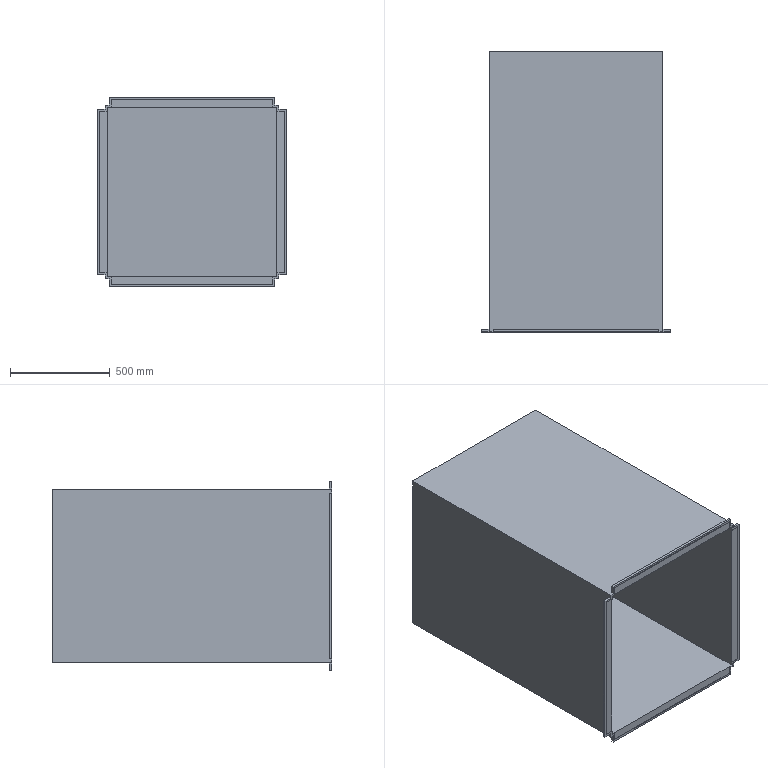Part | SolidWorks | features CirPattern 1, Extrusion 1, ICE 1, RefAxis 1, Shell 1 | 1 solid | 43 faces | box 950 x 1400 x 950 mm | volume 61176455 mm3 | plane 43
STEP:
#1=CARTESIAN_POINT('',(-435.,12.,-415.));
#2=VERTEX_POINT('',#1);
#3=CARTESIAN_POINT('',(-435.,0.,-415.));
#4=VERTEX_POINT('',#3);
#5=CARTESIAN_POINT('',(-435.,1400.,-415.));
#6=DIRECTION('',(0.,-1.,0.));
#7=VECTOR('',#6,1000.);
#8=LINE('',#5,#7);
#9=EDGE_CURVE('',#2,#4,#8,.T.);
#10=ORIENTED_EDGE('',*,*,#9,.F.);
#11=CARTESIAN_POINT('',(-435.,12.,415.));
#12=VERTEX_POINT('',#11);
#13=CARTESIAN_POINT('',(-435.,12.,435.));
#14=DIRECTION('',(0.,0.,-1.));
#15=VECTOR('',#14,1000.);
#16=LINE('',#13,#15);
#17=EDGE_CURVE('',#12,#2,#16,.T.);
#18=ORIENTED_EDGE('',*,*,#17,.F.);
#19=CARTESIAN_POINT('',(-435.,0.,415.));
#20=VERTEX_POINT('',#19);
#21=CARTESIAN_POINT('',(-435.,1400.,415.));
#22=DIRECTION('',(0.,1.,0.));
#23=VECTOR('',#22,1000.);
#24=LINE('',#21,#23);
#25=EDGE_CURVE('',#20,#12,#24,.T.);
#26=ORIENTED_EDGE('',*,*,#25,.F.);
#27=CARTESIAN_POINT('',(-435.,0.,435.));
#28=VERTEX_POINT('',#27);
#29=CARTESIAN_POINT('',(-435.,0.,435.));
#30=DIRECTION('',(0.,0.,1.));
#31=VECTOR('',#30,1000.);
#32=LINE('',#29,#31);
#33=EDGE_CURVE('',#20,#28,#32,.T.);
#34=ORIENTED_EDGE('',*,*,#33,.T.);
#35=CARTESIAN_POINT('',(-435.,1400.,435.));
#36=VERTEX_POINT('',#35);
#37=CARTESIAN_POINT('',(-435.,1400.,435.));
#38=DIRECTION('',(0.,-1.,0.));
#39=VECTOR('',#38,1000.);
#40=LINE('',#37,#39);
#41=EDGE_CURVE('',#36,#28,#40,.T.);
#42=ORIENTED_EDGE('',*,*,#41,.F.);
#43=CARTESIAN_POINT('',(-435.,1400.,-435.));
#44=VERTEX_POINT('',#43);
#45=CARTESIAN_POINT('',(-435.,1400.,435.));
#46=DIRECTION('',(0.,0.,1.));
#47=VECTOR('',#46,1000.);
#48=LINE('',#45,#47);
#49=EDGE_CURVE('',#44,#36,#48,.T.);
#50=ORIENTED_EDGE('',*,*,#49,.F.);
#51=CARTESIAN_POINT('',(-435.,0.,-435.));
#52=VERTEX_POINT('',#51);
#53=CARTESIAN_POINT('',(-435.,1400.,-435.));
#54=DIRECTION('',(0.,-1.,0.));
#55=VECTOR('',#54,1000.);
#56=LINE('',#53,#55);
#57=EDGE_CURVE('',#44,#52,#56,.T.);
#58=ORIENTED_EDGE('',*,*,#57,.T.);
#59=CARTESIAN_POINT('',(-435.,0.,435.));
#60=DIRECTION('',(0.,0.,1.));
#61=VECTOR('',#60,1000.);
#62=LINE('',#59,#61);
#63=EDGE_CURVE('',#52,#4,#62,.T.);
#64=ORIENTED_EDGE('',*,*,#63,.T.);
#65=EDGE_LOOP('',(#10,#18,#26,#34,#42,#50,#58,#64));
#66=FACE_OUTER_BOUND('',#65,.T.);
#67=CARTESIAN_POINT('',(-435.,1400.,435.));
#68=DIRECTION('',(1.,0.,0.));
#69=DIRECTION('',(0.,0.,-1.));
#70=AXIS2_PLACEMENT_3D('',#67,#68,#69);
#71=PLANE('',#70);
#72=ADVANCED_FACE('',(#66),#71,.F.);
#73=CARTESIAN_POINT('',(435.,0.,-415.));
#74=VERTEX_POINT('',#73);
#75=CARTESIAN_POINT('',(435.,12.,-415.));
#76=VERTEX_POINT('',#75);
#77=CARTESIAN_POINT('',(435.,1400.,-415.));
#78=DIRECTION('',(0.,1.,0.));
#79=VECTOR('',#78,1000.);
#80=LINE('',#77,#79);
#81=EDGE_CURVE('',#74,#76,#80,.T.);
#82=ORIENTED_EDGE('',*,*,#81,.F.);
#83=CARTESIAN_POINT('',(435.,0.,-435.));
#84=VERTEX_POINT('',#83);
#85=CARTESIAN_POINT('',(435.,0.,435.));
#86=DIRECTION('',(0.,0.,-1.));
#87=VECTOR('',#86,1000.);
#88=LINE('',#85,#87);
#89=EDGE_CURVE('',#74,#84,#88,.T.);
#90=ORIENTED_EDGE('',*,*,#89,.T.);
#91=CARTESIAN_POINT('',(435.,1400.,-435.));
#92=VERTEX_POINT('',#91);
#93=CARTESIAN_POINT('',(435.,1400.,-435.));
#94=DIRECTION('',(0.,-1.,0.));
#95=VECTOR('',#94,1000.);
#96=LINE('',#93,#95);
#97=EDGE_CURVE('',#92,#84,#96,.T.);
#98=ORIENTED_EDGE('',*,*,#97,.F.);
#99=CARTESIAN_POINT('',(435.,1400.,435.));
#100=VERTEX_POINT('',#99);
#101=CARTESIAN_POINT('',(435.,1400.,435.));
#102=DIRECTION('',(0.,0.,-1.));
#103=VECTOR('',#102,1000.);
#104=LINE('',#101,#103);
#105=EDGE_CURVE('',#100,#92,#104,.T.);
#106=ORIENTED_EDGE('',*,*,#105,.F.);
#107=CARTESIAN_POINT('',(435.,0.,435.));
#108=VERTEX_POINT('',#107);
#109=CARTESIAN_POINT('',(435.,1400.,435.));
#110=DIRECTION('',(0.,-1.,0.));
#111=VECTOR('',#110,1000.);
#112=LINE('',#109,#111);
#113=EDGE_CURVE('',#100,#108,#112,.T.);
#114=ORIENTED_EDGE('',*,*,#113,.T.);
#115=CARTESIAN_POINT('',(435.,0.,415.));
#116=VERTEX_POINT('',#115);
#117=CARTESIAN_POINT('',(435.,0.,435.));
#118=DIRECTION('',(0.,0.,-1.));
#119=VECTOR('',#118,1000.);
#120=LINE('',#117,#119);
#121=EDGE_CURVE('',#108,#116,#120,.T.);
#122=ORIENTED_EDGE('',*,*,#121,.T.);
#123=CARTESIAN_POINT('',(435.,12.,415.));
#124=VERTEX_POINT('',#123);
#125=CARTESIAN_POINT('',(435.,1400.,415.));
#126=DIRECTION('',(0.,-1.,0.));
#127=VECTOR('',#126,1000.);
#128=LINE('',#125,#127);
#129=EDGE_CURVE('',#124,#116,#128,.T.);
#130=ORIENTED_EDGE('',*,*,#129,.F.);
#131=CARTESIAN_POINT('',(435.,12.,435.));
#132=DIRECTION('',(0.,0.,1.));
#133=VECTOR('',#132,1000.);
#134=LINE('',#131,#133);
#135=EDGE_CURVE('',#76,#124,#134,.T.);
#136=ORIENTED_EDGE('',*,*,#135,.F.);
#137=EDGE_LOOP('',(#82,#90,#98,#106,#114,#122,#130,#136));
#138=FACE_OUTER_BOUND('',#137,.T.);
#139=CARTESIAN_POINT('',(435.,1400.,435.));
#140=DIRECTION('',(-1.,0.,0.));
#141=DIRECTION('',(0.,0.,1.));
#142=AXIS2_PLACEMENT_3D('',#139,#140,#141);
#143=PLANE('',#142);
#144=ADVANCED_FACE('',(#138),#143,.F.);
#145=CARTESIAN_POINT('',(-415.,0.,-435.));
#146=VERTEX_POINT('',#145);
#147=CARTESIAN_POINT('',(-415.,12.,-435.));
#148=VERTEX_POINT('',#147);
#149=CARTESIAN_POINT('',(-415.,1400.,-435.));
#150=DIRECTION('',(0.,1.,0.));
#151=VECTOR('',#150,1000.);
#152=LINE('',#149,#151);
#153=EDGE_CURVE('',#146,#148,#152,.T.);
#154=ORIENTED_EDGE('',*,*,#153,.F.);
#155=CARTESIAN_POINT('',(435.,0.,-435.));
#156=DIRECTION('',(-1.,0.,0.));
#157=VECTOR('',#156,1000.);
#158=LINE('',#155,#157);
#159=EDGE_CURVE('',#146,#52,#158,.T.);
#160=ORIENTED_EDGE('',*,*,#159,.T.);
#161=ORIENTED_EDGE('',*,*,#57,.F.);
#162=CARTESIAN_POINT('',(435.,1400.,-435.));
#163=DIRECTION('',(-1.,0.,0.));
#164=VECTOR('',#163,1000.);
#165=LINE('',#162,#164);
#166=EDGE_CURVE('',#92,#44,#165,.T.);
#167=ORIENTED_EDGE('',*,*,#166,.F.);
#168=ORIENTED_EDGE('',*,*,#97,.T.);
#169=CARTESIAN_POINT('',(415.,0.,-435.));
#170=VERTEX_POINT('',#169);
#171=CARTESIAN_POINT('',(435.,0.,-435.));
#172=DIRECTION('',(-1.,0.,0.));
#173=VECTOR('',#172,1000.);
#174=LINE('',#171,#173);
#175=EDGE_CURVE('',#84,#170,#174,.T.);
#176=ORIENTED_EDGE('',*,*,#175,.T.);
#177=CARTESIAN_POINT('',(415.,12.,-435.));
#178=VERTEX_POINT('',#177);
#179=CARTESIAN_POINT('',(415.,1400.,-435.));
#180=DIRECTION('',(0.,-1.,0.));
#181=VECTOR('',#180,1000.);
#182=LINE('',#179,#181);
#183=EDGE_CURVE('',#178,#170,#182,.T.);
#184=ORIENTED_EDGE('',*,*,#183,.F.);
#185=CARTESIAN_POINT('',(435.,12.,-435.));
#186=DIRECTION('',(1.,0.,0.));
#187=VECTOR('',#186,1000.);
#188=LINE('',#185,#187);
#189=EDGE_CURVE('',#148,#178,#188,.T.);
#190=ORIENTED_EDGE('',*,*,#189,.F.);
#191=EDGE_LOOP('',(#154,#160,#161,#167,#168,#176,#184,#190));
#192=FACE_OUTER_BOUND('',#191,.T.);
#193=CARTESIAN_POINT('',(435.,1400.,-435.));
#194=DIRECTION('',(0.,0.,1.));
#195=DIRECTION('',(1.,0.,0.));
#196=AXIS2_PLACEMENT_3D('',#193,#194,#195);
#197=PLANE('',#196);
#198=ADVANCED_FACE('',(#192),#197,.F.);
#199=CARTESIAN_POINT('',(-415.,12.,435.));
#200=VERTEX_POINT('',#199);
#201=CARTESIAN_POINT('',(-415.,0.,435.));
#202=VERTEX_POINT('',#201);
#203=CARTESIAN_POINT('',(-415.,1400.,435.));
#204=DIRECTION('',(0.,-1.,0.));
#205=VECTOR('',#204,1000.);
#206=LINE('',#203,#205);
#207=EDGE_CURVE('',#200,#202,#206,.T.);
#208=ORIENTED_EDGE('',*,*,#207,.F.);
#209=CARTESIAN_POINT('',(415.,12.,435.));
#210=VERTEX_POINT('',#209);
#211=CARTESIAN_POINT('',(435.,12.,435.));
#212=DIRECTION('',(-1.,0.,0.));
#213=VECTOR('',#212,1000.);
#214=LINE('',#211,#213);
#215=EDGE_CURVE('',#210,#200,#214,.T.);
#216=ORIENTED_EDGE('',*,*,#215,.F.);
#217=CARTESIAN_POINT('',(415.,0.,435.));
#218=VERTEX_POINT('',#217);
#219=CARTESIAN_POINT('',(415.,1400.,435.));
#220=DIRECTION('',(0.,1.,0.));
#221=VECTOR('',#220,1000.);
#222=LINE('',#219,#221);
#223=EDGE_CURVE('',#218,#210,#222,.T.);
#224=ORIENTED_EDGE('',*,*,#223,.F.);
#225=CARTESIAN_POINT('',(435.,0.,435.));
#226=DIRECTION('',(1.,0.,0.));
#227=VECTOR('',#226,1000.);
#228=LINE('',#225,#227);
#229=EDGE_CURVE('',#218,#108,#228,.T.);
#230=ORIENTED_EDGE('',*,*,#229,.T.);
#231=ORIENTED_EDGE('',*,*,#113,.F.);
#232=CARTESIAN_POINT('',(435.,1400.,435.));
#233=DIRECTION('',(1.,0.,0.));
#234=VECTOR('',#233,1000.);
#235=LINE('',#232,#234);
#236=EDGE_CURVE('',#36,#100,#235,.T.);
#237=ORIENTED_EDGE('',*,*,#236,.F.);
#238=ORIENTED_EDGE('',*,*,#41,.T.);
#239=CARTESIAN_POINT('',(435.,0.,435.));
#240=DIRECTION('',(1.,0.,0.));
#241=VECTOR('',#240,1000.);
#242=LINE('',#239,#241);
#243=EDGE_CURVE('',#28,#202,#242,.T.);
#244=ORIENTED_EDGE('',*,*,#243,.T.);
#245=EDGE_LOOP('',(#208,#216,#224,#230,#231,#237,#238,#244));
#246=FACE_OUTER_BOUND('',#245,.T.);
#247=CARTESIAN_POINT('',(435.,1400.,435.));
#248=DIRECTION('',(0.,0.,-1.));
#249=DIRECTION('',(-1.,0.,0.));
#250=AXIS2_PLACEMENT_3D('',#247,#248,#249);
#251=PLANE('',#250);
#252=ADVANCED_FACE('',(#246),#251,.F.);
#253=ORIENTED_EDGE('',*,*,#49,.T.);
#254=ORIENTED_EDGE('',*,*,#236,.T.);
#255=ORIENTED_EDGE('',*,*,#105,.T.);
#256=ORIENTED_EDGE('',*,*,#166,.T.);
#257=EDGE_LOOP('',(#253,#254,#255,#256));
#258=FACE_OUTER_BOUND('',#257,.T.);
#259=CARTESIAN_POINT('',(0.,1400.,0.));
#260=DIRECTION('',(0.,1.,0.));
#261=DIRECTION('',(0.,0.,1.));
#262=AXIS2_PLACEMENT_3D('',#259,#260,#261);
#263=PLANE('',#262);
#264=ADVANCED_FACE('',(#258),#263,.T.);
#265=CARTESIAN_POINT('',(-464.2,0.,404.2));
#266=VERTEX_POINT('',#265);
#267=CARTESIAN_POINT('',(-424.2,0.,404.2));
#268=VERTEX_POINT('',#267);
#269=CARTESIAN_POINT('',(-395.,0.,404.2));
#270=DIRECTION('',(1.,0.,0.));
#271=VECTOR('',#270,1000.);
#272=LINE('',#269,#271);
#273=EDGE_CURVE('',#266,#268,#272,.T.);
#274=ORIENTED_EDGE('',*,*,#273,.T.);
#275=CARTESIAN_POINT('',(-424.2,0.,424.2));
#276=VERTEX_POINT('',#275);
#277=CARTESIAN_POINT('',(-424.2,0.,435.));
#278=DIRECTION('',(0.,0.,1.));
#279=VECTOR('',#278,1000.);
#280=LINE('',#277,#279);
#281=EDGE_CURVE('',#268,#276,#280,.T.);
#282=ORIENTED_EDGE('',*,*,#281,.T.);
#283=CARTESIAN_POINT('',(-404.2,0.,424.2));
#284=VERTEX_POINT('',#283);
#285=CARTESIAN_POINT('',(435.,0.,424.2));
#286=DIRECTION('',(1.,0.,0.));
#287=VECTOR('',#286,1000.);
#288=LINE('',#285,#287);
#289=EDGE_CURVE('',#276,#284,#288,.T.);
#290=ORIENTED_EDGE('',*,*,#289,.T.);
#291=CARTESIAN_POINT('',(-404.2,0.,464.2));
#292=VERTEX_POINT('',#291);
#293=CARTESIAN_POINT('',(-404.2,0.,395.));
#294=DIRECTION('',(0.,0.,1.));
#295=VECTOR('',#294,1000.);
#296=LINE('',#293,#295);
#297=EDGE_CURVE('',#284,#292,#296,.T.);
#298=ORIENTED_EDGE('',*,*,#297,.T.);
#299=CARTESIAN_POINT('',(404.2,0.,464.2));
#300=VERTEX_POINT('',#299);
#301=CARTESIAN_POINT('',(415.,0.,464.2));
#302=DIRECTION('',(1.,0.,0.));
#303=VECTOR('',#302,1000.);
#304=LINE('',#301,#303);
#305=EDGE_CURVE('',#292,#300,#304,.T.);
#306=ORIENTED_EDGE('',*,*,#305,.T.);
#307=CARTESIAN_POINT('',(404.2,0.,424.2));
#308=VERTEX_POINT('',#307);
#309=CARTESIAN_POINT('',(404.2,0.,395.));
#310=DIRECTION('',(0.,0.,-1.));
#311=VECTOR('',#310,1000.);
#312=LINE('',#309,#311);
#313=EDGE_CURVE('',#300,#308,#312,.T.);
#314=ORIENTED_EDGE('',*,*,#313,.T.);
#315=CARTESIAN_POINT('',(424.2,0.,424.2));
#316=VERTEX_POINT('',#315);
#317=CARTESIAN_POINT('',(435.,0.,424.2));
#318=DIRECTION('',(1.,0.,0.));
#319=VECTOR('',#318,1000.);
#320=LINE('',#317,#319);
#321=EDGE_CURVE('',#308,#316,#320,.T.);
#322=ORIENTED_EDGE('',*,*,#321,.T.);
#323=CARTESIAN_POINT('',(424.2,0.,404.2));
#324=VERTEX_POINT('',#323);
#325=CARTESIAN_POINT('',(424.2,0.,435.));
#326=DIRECTION('',(0.,0.,-1.));
#327=VECTOR('',#326,1000.);
#328=LINE('',#325,#327);
#329=EDGE_CURVE('',#316,#324,#328,.T.);
#330=ORIENTED_EDGE('',*,*,#329,.T.);
#331=CARTESIAN_POINT('',(464.2,0.,404.2));
#332=VERTEX_POINT('',#331);
#333=CARTESIAN_POINT('',(395.,0.,404.2));
#334=DIRECTION('',(1.,0.,0.));
#335=VECTOR('',#334,1000.);
#336=LINE('',#333,#335);
#337=EDGE_CURVE('',#324,#332,#336,.T.);
#338=ORIENTED_EDGE('',*,*,#337,.T.);
#339=CARTESIAN_POINT('',(464.2,0.,-404.2));
#340=VERTEX_POINT('',#339);
#341=CARTESIAN_POINT('',(464.2,0.,-415.));
#342=DIRECTION('',(0.,0.,-1.));
#343=VECTOR('',#342,1000.);
#344=LINE('',#341,#343);
#345=EDGE_CURVE('',#332,#340,#344,.T.);
#346=ORIENTED_EDGE('',*,*,#345,.T.);
#347=CARTESIAN_POINT('',(424.2,0.,-404.2));
#348=VERTEX_POINT('',#347);
#349=CARTESIAN_POINT('',(395.,0.,-404.2));
#350=DIRECTION('',(-1.,0.,0.));
#351=VECTOR('',#350,1000.);
#352=LINE('',#349,#351);
#353=EDGE_CURVE('',#340,#348,#352,.T.);
#354=ORIENTED_EDGE('',*,*,#353,.T.);
#355=CARTESIAN_POINT('',(424.2,0.,-424.2));
#356=VERTEX_POINT('',#355);
#357=CARTESIAN_POINT('',(424.2,0.,435.));
#358=DIRECTION('',(0.,0.,-1.));
#359=VECTOR('',#358,1000.);
#360=LINE('',#357,#359);
#361=EDGE_CURVE('',#348,#356,#360,.T.);
#362=ORIENTED_EDGE('',*,*,#361,.T.);
#363=CARTESIAN_POINT('',(404.2,0.,-424.2));
#364=VERTEX_POINT('',#363);
#365=CARTESIAN_POINT('',(435.,0.,-424.2));
#366=DIRECTION('',(-1.,0.,0.));
#367=VECTOR('',#366,1000.);
#368=LINE('',#365,#367);
#369=EDGE_CURVE('',#356,#364,#368,.T.);
#370=ORIENTED_EDGE('',*,*,#369,.T.);
#371=CARTESIAN_POINT('',(404.2,0.,-464.2));
#372=VERTEX_POINT('',#371);
#373=CARTESIAN_POINT('',(404.2,0.,-395.));
#374=DIRECTION('',(0.,0.,-1.));
#375=VECTOR('',#374,1000.);
#376=LINE('',#373,#375);
#377=EDGE_CURVE('',#364,#372,#376,.T.);
#378=ORIENTED_EDGE('',*,*,#377,.T.);
#379=CARTESIAN_POINT('',(-404.2,0.,-464.2));
#380=VERTEX_POINT('',#379);
#381=CARTESIAN_POINT('',(-415.,0.,-464.2));
#382=DIRECTION('',(-1.,0.,0.));
#383=VECTOR('',#382,1000.);
#384=LINE('',#381,#383);
#385=EDGE_CURVE('',#372,#380,#384,.T.);
#386=ORIENTED_EDGE('',*,*,#385,.T.);
#387=CARTESIAN_POINT('',(-404.2,0.,-424.2));
#388=VERTEX_POINT('',#387);
#389=CARTESIAN_POINT('',(-404.2,0.,-395.));
#390=DIRECTION('',(0.,0.,1.));
#391=VECTOR('',#390,1000.);
#392=LINE('',#389,#391);
#393=EDGE_CURVE('',#380,#388,#392,.T.);
#394=ORIENTED_EDGE('',*,*,#393,.T.);
#395=CARTESIAN_POINT('',(-424.2,0.,-424.2));
#396=VERTEX_POINT('',#395);
#397=CARTESIAN_POINT('',(435.,0.,-424.2));
#398=DIRECTION('',(-1.,0.,0.));
#399=VECTOR('',#398,1000.);
#400=LINE('',#397,#399);
#401=EDGE_CURVE('',#388,#396,#400,.T.);
#402=ORIENTED_EDGE('',*,*,#401,.T.);
#403=CARTESIAN_POINT('',(-424.2,0.,-404.2));
#404=VERTEX_POINT('',#403);
#405=CARTESIAN_POINT('',(-424.2,0.,435.));
#406=DIRECTION('',(0.,0.,1.));
#407=VECTOR('',#406,1000.);
#408=LINE('',#405,#407);
#409=EDGE_CURVE('',#396,#404,#408,.T.);
#410=ORIENTED_EDGE('',*,*,#409,.T.);
#411=CARTESIAN_POINT('',(-464.2,0.,-404.2));
#412=VERTEX_POINT('',#411);
#413=CARTESIAN_POINT('',(-395.,0.,-404.2));
#414=DIRECTION('',(-1.,0.,0.));
#415=VECTOR('',#414,1000.);
#416=LINE('',#413,#415);
#417=EDGE_CURVE('',#404,#412,#416,.T.);
#418=ORIENTED_EDGE('',*,*,#417,.T.);
#419=CARTESIAN_POINT('',(-464.2,0.,415.));
#420=DIRECTION('',(0.,0.,1.));
#421=VECTOR('',#420,1000.);
#422=LINE('',#419,#421);
#423=EDGE_CURVE('',#412,#266,#422,.T.);
#424=ORIENTED_EDGE('',*,*,#423,.T.);
#425=EDGE_LOOP('',(#274,#282,#290,#298,#306,#314,#322,#330,#338,#346,#354,#362,#370,#378,#386,#394,#402,#410,#418,#424));
#426=FACE_BOUND('',#425,.T.);
#427=ORIENTED_EDGE('',*,*,#33,.F.);
#428=CARTESIAN_POINT('',(-475.,0.,415.));
#429=VERTEX_POINT('',#428);
#430=CARTESIAN_POINT('',(-395.,0.,415.));
#431=DIRECTION('',(1.,0.,0.));
#432=VECTOR('',#431,1000.);
#433=LINE('',#430,#432);
#434=EDGE_CURVE('',#429,#20,#433,.T.);
#435=ORIENTED_EDGE('',*,*,#434,.F.);
#436=CARTESIAN_POINT('',(-475.,0.,-415.));
#437=VERTEX_POINT('',#436);
#438=CARTESIAN_POINT('',(-475.,0.,415.));
#439=DIRECTION('',(0.,0.,1.));
#440=VECTOR('',#439,1000.);
#441=LINE('',#438,#440);
#442=EDGE_CURVE('',#437,#429,#441,.T.);
#443=ORIENTED_EDGE('',*,*,#442,.F.);
#444=CARTESIAN_POINT('',(-395.,0.,-415.));
#445=DIRECTION('',(-1.,0.,0.));
#446=VECTOR('',#445,1000.);
#447=LINE('',#444,#446);
#448=EDGE_CURVE('',#4,#437,#447,.T.);
#449=ORIENTED_EDGE('',*,*,#448,.F.);
#450=ORIENTED_EDGE('',*,*,#63,.F.);
#451=ORIENTED_EDGE('',*,*,#159,.F.);
#452=CARTESIAN_POINT('',(-415.,0.,-475.));
#453=VERTEX_POINT('',#452);
#454=CARTESIAN_POINT('',(-415.,0.,-395.));
#455=DIRECTION('',(0.,0.,1.));
#456=VECTOR('',#455,1000.);
#457=LINE('',#454,#456);
#458=EDGE_CURVE('',#453,#146,#457,.T.);
#459=ORIENTED_EDGE('',*,*,#458,.F.);
#460=CARTESIAN_POINT('',(415.,0.,-475.));
#461=VERTEX_POINT('',#460);
#462=CARTESIAN_POINT('',(-415.,0.,-475.));
#463=DIRECTION('',(-1.,0.,0.));
#464=VECTOR('',#463,1000.);
#465=LINE('',#462,#464);
#466=EDGE_CURVE('',#461,#453,#465,.T.);
#467=ORIENTED_EDGE('',*,*,#466,.F.);
#468=CARTESIAN_POINT('',(415.,0.,-395.));
#469=DIRECTION('',(0.,0.,-1.));
#470=VECTOR('',#469,1000.);
#471=LINE('',#468,#470);
#472=EDGE_CURVE('',#170,#461,#471,.T.);
#473=ORIENTED_EDGE('',*,*,#472,.F.);
#474=ORIENTED_EDGE('',*,*,#175,.F.);
#475=ORIENTED_EDGE('',*,*,#89,.F.);
#476=CARTESIAN_POINT('',(475.,0.,-415.));
#477=VERTEX_POINT('',#476);
#478=CARTESIAN_POINT('',(395.,0.,-415.));
#479=DIRECTION('',(-1.,0.,0.));
#480=VECTOR('',#479,1000.);
#481=LINE('',#478,#480);
#482=EDGE_CURVE('',#477,#74,#481,.T.);
#483=ORIENTED_EDGE('',*,*,#482,.F.);
#484=CARTESIAN_POINT('',(475.,0.,415.));
#485=VERTEX_POINT('',#484);
#486=CARTESIAN_POINT('',(475.,0.,-415.));
#487=DIRECTION('',(0.,0.,-1.));
#488=VECTOR('',#487,1000.);
#489=LINE('',#486,#488);
#490=EDGE_CURVE('',#485,#477,#489,.T.);
#491=ORIENTED_EDGE('',*,*,#490,.F.);
#492=CARTESIAN_POINT('',(395.,0.,415.));
#493=DIRECTION('',(1.,0.,0.));
#494=VECTOR('',#493,1000.);
#495=LINE('',#492,#494);
#496=EDGE_CURVE('',#116,#485,#495,.T.);
#497=ORIENTED_EDGE('',*,*,#496,.F.);
#498=ORIENTED_EDGE('',*,*,#121,.F.);
#499=ORIENTED_EDGE('',*,*,#229,.F.);
#500=CARTESIAN_POINT('',(415.,0.,475.));
#501=VERTEX_POINT('',#500);
#502=CARTESIAN_POINT('',(415.,0.,395.));
#503=DIRECTION('',(0.,0.,-1.));
#504=VECTOR('',#503,1000.);
#505=LINE('',#502,#504);
#506=EDGE_CURVE('',#501,#218,#505,.T.);
#507=ORIENTED_EDGE('',*,*,#506,.F.);
#508=CARTESIAN_POINT('',(-415.,0.,475.));
#509=VERTEX_POINT('',#508);
#510=CARTESIAN_POINT('',(415.,0.,475.));
#511=DIRECTION('',(1.,0.,0.));
#512=VECTOR('',#511,1000.);
#513=LINE('',#510,#512);
#514=EDGE_CURVE('',#509,#501,#513,.T.);
#515=ORIENTED_EDGE('',*,*,#514,.F.);
#516=CARTESIAN_POINT('',(-415.,0.,395.));
#517=DIRECTION('',(0.,0.,1.));
#518=VECTOR('',#517,1000.);
#519=LINE('',#516,#518);
#520=EDGE_CURVE('',#202,#509,#519,.T.);
#521=ORIENTED_EDGE('',*,*,#520,.F.);
#522=ORIENTED_EDGE('',*,*,#243,.F.);
#523=EDGE_LOOP('',(#427,#435,#443,#449,#450,#451,#459,#467,#473,#474,#475,#483,#491,#497,#498,#499,#507,#515,#521,#522));
#524=FACE_OUTER_BOUND('',#523,.T.);
#525=CARTESIAN_POINT('',(0.,0.,0.));
#526=DIRECTION('',(0.,1.,0.));
#527=DIRECTION('',(0.,0.,1.));
#528=AXIS2_PLACEMENT_3D('',#525,#526,#527);
#529=PLANE('',#528);
#530=ADVANCED_FACE('',(#426,#524),#529,.F.);
#531=CARTESIAN_POINT('',(415.,12.,475.));
#532=VERTEX_POINT('',#531);
#533=CARTESIAN_POINT('',(415.,12.,395.));
#534=DIRECTION('',(0.,0.,-1.));
#535=VECTOR('',#534,1000.);
#536=LINE('',#533,#535);
#537=EDGE_CURVE('',#532,#210,#536,.T.);
#538=ORIENTED_EDGE('',*,*,#537,.T.);
#539=ORIENTED_EDGE('',*,*,#215,.T.);
#540=CARTESIAN_POINT('',(-415.,12.,475.));
#541=VERTEX_POINT('',#540);
#542=CARTESIAN_POINT('',(-415.,12.,395.));
#543=DIRECTION('',(0.,0.,1.));
#544=VECTOR('',#543,1000.);
#545=LINE('',#542,#544);
#546=EDGE_CURVE('',#200,#541,#545,.T.);
#547=ORIENTED_EDGE('',*,*,#546,.T.);
#548=CARTESIAN_POINT('',(415.,12.,475.));
#549=DIRECTION('',(1.,0.,0.));
#550=VECTOR('',#549,1000.);
#551=LINE('',#548,#550);
#552=EDGE_CURVE('',#541,#532,#551,.T.);
#553=ORIENTED_EDGE('',*,*,#552,.T.);
#554=EDGE_LOOP('',(#538,#539,#547,#553));
#555=FACE_OUTER_BOUND('',#554,.T.);
#556=CARTESIAN_POINT('',(0.,12.,0.));
#557=DIRECTION('',(0.,-1.,0.));
#558=DIRECTION('',(0.,0.,-1.));
#559=AXIS2_PLACEMENT_3D('',#556,#557,#558);
#560=PLANE('',#559);
#561=ADVANCED_FACE('',(#555),#560,.F.);
#562=ORIENTED_EDGE('',*,*,#546,.F.);
#563=ORIENTED_EDGE('',*,*,#207,.T.);
#564=ORIENTED_EDGE('',*,*,#520,.T.);
#565=CARTESIAN_POINT('',(-415.,12.,475.));
#566=DIRECTION('',(0.,-1.,0.));
#567=VECTOR('',#566,1000.);
#568=LINE('',#565,#567);
#569=EDGE_CURVE('',#541,#509,#568,.T.);
#570=ORIENTED_EDGE('',*,*,#569,.F.);
#571=EDGE_LOOP('',(#562,#563,#564,#570));
#572=FACE_OUTER_BOUND('',#571,.T.);
#573=CARTESIAN_POINT('',(-415.,12.,395.));
#574=DIRECTION('',(1.,0.,0.));
#575=DIRECTION('',(0.,0.,-1.));
#576=AXIS2_PLACEMENT_3D('',#573,#574,#575);
#577=PLANE('',#576);
#578=ADVANCED_FACE('',(#572),#577,.F.);
#579=ORIENTED_EDGE('',*,*,#506,.T.);
#580=ORIENTED_EDGE('',*,*,#223,.T.);
#581=ORIENTED_EDGE('',*,*,#537,.F.);
#582=CARTESIAN_POINT('',(415.,12.,475.));
#583=DIRECTION('',(0.,-1.,0.));
#584=VECTOR('',#583,1000.);
#585=LINE('',#582,#584);
#586=EDGE_CURVE('',#532,#501,#585,.T.);
#587=ORIENTED_EDGE('',*,*,#586,.T.);
#588=EDGE_LOOP('',(#579,#580,#581,#587));
#589=FACE_OUTER_BOUND('',#588,.T.);
#590=CARTESIAN_POINT('',(415.,12.,395.));
#591=DIRECTION('',(-1.,0.,0.));
#592=DIRECTION('',(0.,0.,1.));
#593=AXIS2_PLACEMENT_3D('',#590,#591,#592);
#594=PLANE('',#593);
#595=ADVANCED_FACE('',(#589),#594,.F.);
#596=ORIENTED_EDGE('',*,*,#514,.T.);
#597=ORIENTED_EDGE('',*,*,#586,.F.);
#598=ORIENTED_EDGE('',*,*,#552,.F.);
#599=ORIENTED_EDGE('',*,*,#569,.T.);
#600=EDGE_LOOP('',(#596,#597,#598,#599));
#601=FACE_OUTER_BOUND('',#600,.T.);
#602=CARTESIAN_POINT('',(415.,12.,475.));
#603=DIRECTION('',(0.,0.,-1.));
#604=DIRECTION('',(-1.,0.,0.));
#605=AXIS2_PLACEMENT_3D('',#602,#603,#604);
#606=PLANE('',#605);
#607=ADVANCED_FACE('',(#601),#606,.F.);
#608=ORIENTED_EDGE('',*,*,#466,.T.);
#609=CARTESIAN_POINT('',(-415.,12.,-475.));
#610=VERTEX_POINT('',#609);
#611=CARTESIAN_POINT('',(-415.,12.,-475.));
#612=DIRECTION('',(0.,-1.,0.));
#613=VECTOR('',#612,1000.);
#614=LINE('',#611,#613);
#615=EDGE_CURVE('',#610,#453,#614,.T.);
#616=ORIENTED_EDGE('',*,*,#615,.F.);
#617=CARTESIAN_POINT('',(415.,12.,-475.));
#618=VERTEX_POINT('',#617);
#619=CARTESIAN_POINT('',(-415.,12.,-475.));
#620=DIRECTION('',(-1.,0.,0.));
#621=VECTOR('',#620,1000.);
#622=LINE('',#619,#621);
#623=EDGE_CURVE('',#618,#610,#622,.T.);
#624=ORIENTED_EDGE('',*,*,#623,.F.);
#625=CARTESIAN_POINT('',(415.,12.,-475.));
#626=DIRECTION('',(0.,-1.,0.));
#627=VECTOR('',#626,1000.);
#628=LINE('',#625,#627);
#629=EDGE_CURVE('',#618,#461,#628,.T.);
#630=ORIENTED_EDGE('',*,*,#629,.T.);
#631=EDGE_LOOP('',(#608,#616,#624,#630));
#632=FACE_OUTER_BOUND('',#631,.T.);
#633=CARTESIAN_POINT('',(-415.,12.,-475.));
#634=DIRECTION('',(0.,0.,1.));
#635=DIRECTION('',(1.,0.,0.));
#636=AXIS2_PLACEMENT_3D('',#633,#634,#635);
#637=PLANE('',#636);
#638=ADVANCED_FACE('',(#632),#637,.F.);
#639=CARTESIAN_POINT('',(415.,12.,-395.));
#640=DIRECTION('',(0.,0.,-1.));
#641=VECTOR('',#640,1000.);
#642=LINE('',#639,#641);
#643=EDGE_CURVE('',#178,#618,#642,.T.);
#644=ORIENTED_EDGE('',*,*,#643,.F.);
#645=ORIENTED_EDGE('',*,*,#183,.T.);
#646=ORIENTED_EDGE('',*,*,#472,.T.);
#647=ORIENTED_EDGE('',*,*,#629,.F.);
#648=EDGE_LOOP('',(#644,#645,#646,#647));
#649=FACE_OUTER_BOUND('',#648,.T.);
#650=CARTESIAN_POINT('',(415.,12.,-395.));
#651=DIRECTION('',(-1.,0.,0.));
#652=DIRECTION('',(0.,0.,1.));
#653=AXIS2_PLACEMENT_3D('',#650,#651,#652);
#654=PLANE('',#653);
#655=ADVANCED_FACE('',(#649),#654,.F.);
#656=ORIENTED_EDGE('',*,*,#458,.T.);
#657=ORIENTED_EDGE('',*,*,#153,.T.);
#658=CARTESIAN_POINT('',(-415.,12.,-395.));
#659=DIRECTION('',(0.,0.,1.));
#660=VECTOR('',#659,1000.);
#661=LINE('',#658,#660);
#662=EDGE_CURVE('',#610,#148,#661,.T.);
#663=ORIENTED_EDGE('',*,*,#662,.F.);
#664=ORIENTED_EDGE('',*,*,#615,.T.);
#665=EDGE_LOOP('',(#656,#657,#663,#664));
#666=FACE_OUTER_BOUND('',#665,.T.);
#667=CARTESIAN_POINT('',(-415.,12.,-395.));
#668=DIRECTION('',(1.,0.,0.));
#669=DIRECTION('',(0.,0.,-1.));
#670=AXIS2_PLACEMENT_3D('',#667,#668,#669);
#671=PLANE('',#670);
#672=ADVANCED_FACE('',(#666),#671,.F.);
#673=ORIENTED_EDGE('',*,*,#662,.T.);
#674=ORIENTED_EDGE('',*,*,#189,.T.);
#675=ORIENTED_EDGE('',*,*,#643,.T.);
#676=ORIENTED_EDGE('',*,*,#623,.T.);
#677=EDGE_LOOP('',(#673,#674,#675,#676));
#678=FACE_OUTER_BOUND('',#677,.T.);
#679=CARTESIAN_POINT('',(0.,12.,0.));
#680=DIRECTION('',(0.,-1.,0.));
#681=DIRECTION('',(1.,0.,0.));
#682=AXIS2_PLACEMENT_3D('',#679,#680,#681);
#683=PLANE('',#682);
#684=ADVANCED_FACE('',(#678),#683,.F.);
#685=ORIENTED_EDGE('',*,*,#490,.T.);
#686=CARTESIAN_POINT('',(475.,12.,-415.));
#687=VERTEX_POINT('',#686);
#688=CARTESIAN_POINT('',(475.,12.,-415.));
#689=DIRECTION('',(0.,-1.,0.));
#690=VECTOR('',#689,1000.);
#691=LINE('',#688,#690);
#692=EDGE_CURVE('',#687,#477,#691,.T.);
#693=ORIENTED_EDGE('',*,*,#692,.F.);
#694=CARTESIAN_POINT('',(475.,12.,415.));
#695=VERTEX_POINT('',#694);
#696=CARTESIAN_POINT('',(475.,12.,-415.));
#697=DIRECTION('',(0.,0.,-1.));
#698=VECTOR('',#697,1000.);
#699=LINE('',#696,#698);
#700=EDGE_CURVE('',#695,#687,#699,.T.);
#701=ORIENTED_EDGE('',*,*,#700,.F.);
#702=CARTESIAN_POINT('',(475.,12.,415.));
#703=DIRECTION('',(0.,-1.,0.));
#704=VECTOR('',#703,1000.);
#705=LINE('',#702,#704);
#706=EDGE_CURVE('',#695,#485,#705,.T.);
#707=ORIENTED_EDGE('',*,*,#706,.T.);
#708=EDGE_LOOP('',(#685,#693,#701,#707));
#709=FACE_OUTER_BOUND('',#708,.T.);
#710=CARTESIAN_POINT('',(475.,12.,-415.));
#711=DIRECTION('',(-1.,0.,0.));
#712=DIRECTION('',(0.,0.,1.));
#713=AXIS2_PLACEMENT_3D('',#710,#711,#712);
#714=PLANE('',#713);
#715=ADVANCED_FACE('',(#709),#714,.F.);
#716=CARTESIAN_POINT('',(395.,12.,415.));
#717=DIRECTION('',(1.,0.,0.));
#718=VECTOR('',#717,1000.);
#719=LINE('',#716,#718);
#720=EDGE_CURVE('',#124,#695,#719,.T.);
#721=ORIENTED_EDGE('',*,*,#720,.F.);
#722=ORIENTED_EDGE('',*,*,#129,.T.);
#723=ORIENTED_EDGE('',*,*,#496,.T.);
#724=ORIENTED_EDGE('',*,*,#706,.F.);
#725=EDGE_LOOP('',(#721,#722,#723,#724));
#726=FACE_OUTER_BOUND('',#725,.T.);
#727=CARTESIAN_POINT('',(395.,12.,415.));
#728=DIRECTION('',(0.,0.,-1.));
#729=DIRECTION('',(-1.,0.,0.));
#730=AXIS2_PLACEMENT_3D('',#727,#728,#729);
#731=PLANE('',#730);
#732=ADVANCED_FACE('',(#726),#731,.F.);
#733=ORIENTED_EDGE('',*,*,#482,.T.);
#734=ORIENTED_EDGE('',*,*,#81,.T.);
#735=CARTESIAN_POINT('',(395.,12.,-415.));
#736=DIRECTION('',(-1.,0.,0.));
#737=VECTOR('',#736,1000.);
#738=LINE('',#735,#737);
#739=EDGE_CURVE('',#687,#76,#738,.T.);
#740=ORIENTED_EDGE('',*,*,#739,.F.);
#741=ORIENTED_EDGE('',*,*,#692,.T.);
#742=EDGE_LOOP('',(#733,#734,#740,#741));
#743=FACE_OUTER_BOUND('',#742,.T.);
#744=CARTESIAN_POINT('',(395.,12.,-415.));
#745=DIRECTION('',(0.,0.,1.));
#746=DIRECTION('',(1.,0.,0.));
#747=AXIS2_PLACEMENT_3D('',#744,#745,#746);
#748=PLANE('',#747);
#749=ADVANCED_FACE('',(#743),#748,.F.);
#750=ORIENTED_EDGE('',*,*,#739,.T.);
#751=ORIENTED_EDGE('',*,*,#135,.T.);
#752=ORIENTED_EDGE('',*,*,#720,.T.);
#753=ORIENTED_EDGE('',*,*,#700,.T.);
#754=EDGE_LOOP('',(#750,#751,#752,#753));
#755=FACE_OUTER_BOUND('',#754,.T.);
#756=CARTESIAN_POINT('',(0.,12.,0.));
#757=DIRECTION('',(0.,-1.,0.));
#758=DIRECTION('',(1.,0.,0.));
#759=AXIS2_PLACEMENT_3D('',#756,#757,#758);
#760=PLANE('',#759);
#761=ADVANCED_FACE('',(#755),#760,.F.);
#762=CARTESIAN_POINT('',(-475.,12.,415.));
#763=VERTEX_POINT('',#762);
#764=CARTESIAN_POINT('',(-395.,12.,415.));
#765=DIRECTION('',(1.,0.,0.));
#766=VECTOR('',#765,1000.);
#767=LINE('',#764,#766);
#768=EDGE_CURVE('',#763,#12,#767,.T.);
#769=ORIENTED_EDGE('',*,*,#768,.T.);
#770=ORIENTED_EDGE('',*,*,#17,.T.);
#771=CARTESIAN_POINT('',(-475.,12.,-415.));
#772=VERTEX_POINT('',#771);
#773=CARTESIAN_POINT('',(-395.,12.,-415.));
#774=DIRECTION('',(-1.,0.,0.));
#775=VECTOR('',#774,1000.);
#776=LINE('',#773,#775);
#777=EDGE_CURVE('',#2,#772,#776,.T.);
#778=ORIENTED_EDGE('',*,*,#777,.T.);
#779=CARTESIAN_POINT('',(-475.,12.,415.));
#780=DIRECTION('',(0.,0.,1.));
#781=VECTOR('',#780,1000.);
#782=LINE('',#779,#781);
#783=EDGE_CURVE('',#772,#763,#782,.T.);
#784=ORIENTED_EDGE('',*,*,#783,.T.);
#785=EDGE_LOOP('',(#769,#770,#778,#784));
#786=FACE_OUTER_BOUND('',#785,.T.);
#787=CARTESIAN_POINT('',(0.,12.,0.));
#788=DIRECTION('',(0.,-1.,0.));
#789=DIRECTION('',(1.,0.,0.));
#790=AXIS2_PLACEMENT_3D('',#787,#788,#789);
#791=PLANE('',#790);
#792=ADVANCED_FACE('',(#786),#791,.F.);
#793=ORIENTED_EDGE('',*,*,#777,.F.);
#794=ORIENTED_EDGE('',*,*,#9,.T.);
#795=ORIENTED_EDGE('',*,*,#448,.T.);
#796=CARTESIAN_POINT('',(-475.,12.,-415.));
#797=DIRECTION('',(0.,-1.,0.));
#798=VECTOR('',#797,1000.);
#799=LINE('',#796,#798);
#800=EDGE_CURVE('',#772,#437,#799,.T.);
#801=ORIENTED_EDGE('',*,*,#800,.F.);
#802=EDGE_LOOP('',(#793,#794,#795,#801));
#803=FACE_OUTER_BOUND('',#802,.T.);
#804=CARTESIAN_POINT('',(-395.,12.,-415.));
#805=DIRECTION('',(0.,0.,1.));
#806=DIRECTION('',(1.,0.,0.));
#807=AXIS2_PLACEMENT_3D('',#804,#805,#806);
#808=PLANE('',#807);
#809=ADVANCED_FACE('',(#803),#808,.F.);
#810=ORIENTED_EDGE('',*,*,#434,.T.);
#811=ORIENTED_EDGE('',*,*,#25,.T.);
#812=ORIENTED_EDGE('',*,*,#768,.F.);
#813=CARTESIAN_POINT('',(-475.,12.,415.));
#814=DIRECTION('',(0.,-1.,0.));
#815=VECTOR('',#814,1000.);
#816=LINE('',#813,#815);
#817=EDGE_CURVE('',#763,#429,#816,.T.);
#818=ORIENTED_EDGE('',*,*,#817,.T.);
#819=EDGE_LOOP('',(#810,#811,#812,#818));
#820=FACE_OUTER_BOUND('',#819,.T.);
#821=CARTESIAN_POINT('',(-395.,12.,415.));
#822=DIRECTION('',(0.,0.,-1.));
#823=DIRECTION('',(-1.,0.,0.));
#824=AXIS2_PLACEMENT_3D('',#821,#822,#823);
#825=PLANE('',#824);
#826=ADVANCED_FACE('',(#820),#825,.F.);
#827=ORIENTED_EDGE('',*,*,#442,.T.);
#828=ORIENTED_EDGE('',*,*,#817,.F.);
#829=ORIENTED_EDGE('',*,*,#783,.F.);
#830=ORIENTED_EDGE('',*,*,#800,.T.);
#831=EDGE_LOOP('',(#827,#828,#829,#830));
#832=FACE_OUTER_BOUND('',#831,.T.);
#833=CARTESIAN_POINT('',(-475.,12.,415.));
#834=DIRECTION('',(1.,0.,0.));
#835=DIRECTION('',(0.,0.,-1.));
#836=AXIS2_PLACEMENT_3D('',#833,#834,#835);
#837=PLANE('',#836);
#838=ADVANCED_FACE('',(#832),#837,.F.);
#839=CARTESIAN_POINT('',(-424.2,1.2,-404.2));
#840=VERTEX_POINT('',#839);
#841=CARTESIAN_POINT('',(-424.2,1400.,-404.2));
#842=DIRECTION('',(0.,-1.,0.));
#843=VECTOR('',#842,1000.);
#844=LINE('',#841,#843);
#845=EDGE_CURVE('',#840,#404,#844,.T.);
#846=ORIENTED_EDGE('',*,*,#845,.T.);
#847=ORIENTED_EDGE('',*,*,#409,.F.);
#848=CARTESIAN_POINT('',(-424.2,1389.2,-424.2));
#849=VERTEX_POINT('',#848);
#850=CARTESIAN_POINT('',(-424.2,1400.,-424.2));
#851=DIRECTION('',(0.,-1.,0.));
#852=VECTOR('',#851,1000.);
#853=LINE('',#850,#852);
#854=EDGE_CURVE('',#849,#396,#853,.T.);
#855=ORIENTED_EDGE('',*,*,#854,.F.);
#856=CARTESIAN_POINT('',(-424.2,1389.2,424.2));
#857=VERTEX_POINT('',#856);
#858=CARTESIAN_POINT('',(-424.2,1389.2,435.));
#859=DIRECTION('',(0.,0.,1.));
#860=VECTOR('',#859,1000.);
#861=LINE('',#858,#860);
#862=EDGE_CURVE('',#849,#857,#861,.T.);
#863=ORIENTED_EDGE('',*,*,#862,.T.);
#864=CARTESIAN_POINT('',(-424.2,1400.,424.2));
#865=DIRECTION('',(0.,-1.,0.));
#866=VECTOR('',#865,1000.);
#867=LINE('',#864,#866);
#868=EDGE_CURVE('',#857,#276,#867,.T.);
#869=ORIENTED_EDGE('',*,*,#868,.T.);
#870=ORIENTED_EDGE('',*,*,#281,.F.);
#871=CARTESIAN_POINT('',(-424.2,1.2,404.2));
#872=VERTEX_POINT('',#871);
#873=CARTESIAN_POINT('',(-424.2,1400.,404.2));
#874=DIRECTION('',(0.,1.,0.));
#875=VECTOR('',#874,1000.);
#876=LINE('',#873,#875);
#877=EDGE_CURVE('',#268,#872,#876,.T.);
#878=ORIENTED_EDGE('',*,*,#877,.T.);
#879=CARTESIAN_POINT('',(-424.2,1.2,435.));
#880=DIRECTION('',(0.,0.,-1.));
#881=VECTOR('',#880,1000.);
#882=LINE('',#879,#881);
#883=EDGE_CURVE('',#872,#840,#882,.T.);
#884=ORIENTED_EDGE('',*,*,#883,.T.);
#885=EDGE_LOOP('',(#846,#847,#855,#863,#869,#870,#878,#884));
#886=FACE_OUTER_BOUND('',#885,.T.);
#887=CARTESIAN_POINT('',(-424.2,1400.,435.));
#888=DIRECTION('',(1.,0.,0.));
#889=DIRECTION('',(0.,0.,-1.));
#890=AXIS2_PLACEMENT_3D('',#887,#888,#889);
#891=PLANE('',#890);
#892=ADVANCED_FACE('',(#886),#891,.T.);
#893=CARTESIAN_POINT('',(424.2,1.2,-404.2));
#894=VERTEX_POINT('',#893);
#895=CARTESIAN_POINT('',(424.2,1400.,-404.2));
#896=DIRECTION('',(0.,1.,0.));
#897=VECTOR('',#896,1000.);
#898=LINE('',#895,#897);
#899=EDGE_CURVE('',#348,#894,#898,.T.);
#900=ORIENTED_EDGE('',*,*,#899,.T.);
#901=CARTESIAN_POINT('',(424.2,1.2,404.2));
#902=VERTEX_POINT('',#901);
#903=CARTESIAN_POINT('',(424.2,1.2,435.));
#904=DIRECTION('',(0.,0.,1.));
#905=VECTOR('',#904,1000.);
#906=LINE('',#903,#905);
#907=EDGE_CURVE('',#894,#902,#906,.T.);
#908=ORIENTED_EDGE('',*,*,#907,.T.);
#909=CARTESIAN_POINT('',(424.2,1400.,404.2));
#910=DIRECTION('',(0.,-1.,0.));
#911=VECTOR('',#910,1000.);
#912=LINE('',#909,#911);
#913=EDGE_CURVE('',#902,#324,#912,.T.);
#914=ORIENTED_EDGE('',*,*,#913,.T.);
#915=ORIENTED_EDGE('',*,*,#329,.F.);
#916=CARTESIAN_POINT('',(424.2,1389.2,424.2));
#917=VERTEX_POINT('',#916);
#918=CARTESIAN_POINT('',(424.2,1400.,424.2));
#919=DIRECTION('',(0.,-1.,0.));
#920=VECTOR('',#919,1000.);
#921=LINE('',#918,#920);
#922=EDGE_CURVE('',#917,#316,#921,.T.);
#923=ORIENTED_EDGE('',*,*,#922,.F.);
#924=CARTESIAN_POINT('',(424.2,1389.2,-424.2));
#925=VERTEX_POINT('',#924);
#926=CARTESIAN_POINT('',(424.2,1389.2,435.));
#927=DIRECTION('',(0.,0.,-1.));
#928=VECTOR('',#927,1000.);
#929=LINE('',#926,#928);
#930=EDGE_CURVE('',#917,#925,#929,.T.);
#931=ORIENTED_EDGE('',*,*,#930,.T.);
#932=CARTESIAN_POINT('',(424.2,1400.,-424.2));
#933=DIRECTION('',(0.,-1.,0.));
#934=VECTOR('',#933,1000.);
#935=LINE('',#932,#934);
#936=EDGE_CURVE('',#925,#356,#935,.T.);
#937=ORIENTED_EDGE('',*,*,#936,.T.);
#938=ORIENTED_EDGE('',*,*,#361,.F.);
#939=EDGE_LOOP('',(#900,#908,#914,#915,#923,#931,#937,#938));
#940=FACE_OUTER_BOUND('',#939,.T.);
#941=CARTESIAN_POINT('',(424.2,1400.,435.));
#942=DIRECTION('',(-1.,0.,0.));
#943=DIRECTION('',(0.,0.,1.));
#944=AXIS2_PLACEMENT_3D('',#941,#942,#943);
#945=PLANE('',#944);
#946=ADVANCED_FACE('',(#940),#945,.T.);
#947=CARTESIAN_POINT('',(-404.2,1.2,-424.2));
#948=VERTEX_POINT('',#947);
#949=CARTESIAN_POINT('',(-404.2,1400.,-424.2));
#950=DIRECTION('',(0.,1.,0.));
#951=VECTOR('',#950,1000.);
#952=LINE('',#949,#951);
#953=EDGE_CURVE('',#388,#948,#952,.T.);
#954=ORIENTED_EDGE('',*,*,#953,.T.);
#955=CARTESIAN_POINT('',(404.2,1.2,-424.2));
#956=VERTEX_POINT('',#955);
#957=CARTESIAN_POINT('',(435.,1.2,-424.2));
#958=DIRECTION('',(1.,0.,0.));
#959=VECTOR('',#958,1000.);
#960=LINE('',#957,#959);
#961=EDGE_CURVE('',#948,#956,#960,.T.);
#962=ORIENTED_EDGE('',*,*,#961,.T.);
#963=CARTESIAN_POINT('',(404.2,1400.,-424.2));
#964=DIRECTION('',(0.,-1.,0.));
#965=VECTOR('',#964,1000.);
#966=LINE('',#963,#965);
#967=EDGE_CURVE('',#956,#364,#966,.T.);
#968=ORIENTED_EDGE('',*,*,#967,.T.);
#969=ORIENTED_EDGE('',*,*,#369,.F.);
#970=ORIENTED_EDGE('',*,*,#936,.F.);
#971=CARTESIAN_POINT('',(435.,1389.2,-424.2));
#972=DIRECTION('',(-1.,0.,0.));
#973=VECTOR('',#972,1000.);
#974=LINE('',#971,#973);
#975=EDGE_CURVE('',#925,#849,#974,.T.);
#976=ORIENTED_EDGE('',*,*,#975,.T.);
#977=ORIENTED_EDGE('',*,*,#854,.T.);
#978=ORIENTED_EDGE('',*,*,#401,.F.);
#979=EDGE_LOOP('',(#954,#962,#968,#969,#970,#976,#977,#978));
#980=FACE_OUTER_BOUND('',#979,.T.);
#981=CARTESIAN_POINT('',(435.,1400.,-424.2));
#982=DIRECTION('',(0.,0.,1.));
#983=DIRECTION('',(1.,0.,0.));
#984=AXIS2_PLACEMENT_3D('',#981,#982,#983);
#985=PLANE('',#984);
#986=ADVANCED_FACE('',(#980),#985,.T.);
#987=CARTESIAN_POINT('',(-404.2,1.2,424.2));
#988=VERTEX_POINT('',#987);
#989=CARTESIAN_POINT('',(-404.2,1400.,424.2));
#990=DIRECTION('',(0.,-1.,0.));
#991=VECTOR('',#990,1000.);
#992=LINE('',#989,#991);
#993=EDGE_CURVE('',#988,#284,#992,.T.);
#994=ORIENTED_EDGE('',*,*,#993,.T.);
#995=ORIENTED_EDGE('',*,*,#289,.F.);
#996=ORIENTED_EDGE('',*,*,#868,.F.);
#997=CARTESIAN_POINT('',(435.,1389.2,424.2));
#998=DIRECTION('',(1.,0.,0.));
#999=VECTOR('',#998,1000.);
#1000=LINE('',#997,#999);
#1001=EDGE_CURVE('',#857,#917,#1000,.T.);
#1002=ORIENTED_EDGE('',*,*,#1001,.T.);
#1003=ORIENTED_EDGE('',*,*,#922,.T.);
#1004=ORIENTED_EDGE('',*,*,#321,.F.);
#1005=CARTESIAN_POINT('',(404.2,1.2,424.2));
#1006=VERTEX_POINT('',#1005);
#1007=CARTESIAN_POINT('',(404.2,1400.,424.2));
#1008=DIRECTION('',(0.,1.,0.));
#1009=VECTOR('',#1008,1000.);
#1010=LINE('',#1007,#1009);
#1011=EDGE_CURVE('',#308,#1006,#1010,.T.);
#1012=ORIENTED_EDGE('',*,*,#1011,.T.);
#1013=CARTESIAN_POINT('',(435.,1.2,424.2));
#1014=DIRECTION('',(-1.,0.,0.));
#1015=VECTOR('',#1014,1000.);
#1016=LINE('',#1013,#1015);
#1017=EDGE_CURVE('',#1006,#988,#1016,.T.);
#1018=ORIENTED_EDGE('',*,*,#1017,.T.);
#1019=EDGE_LOOP('',(#994,#995,#996,#1002,#1003,#1004,#1012,#1018));
#1020=FACE_OUTER_BOUND('',#1019,.T.);
#1021=CARTESIAN_POINT('',(435.,1400.,424.2));
#1022=DIRECTION('',(0.,0.,-1.));
#1023=DIRECTION('',(-1.,0.,0.));
#1024=AXIS2_PLACEMENT_3D('',#1021,#1022,#1023);
#1025=PLANE('',#1024);
#1026=ADVANCED_FACE('',(#1020),#1025,.T.);
#1027=ORIENTED_EDGE('',*,*,#862,.F.);
#1028=ORIENTED_EDGE('',*,*,#975,.F.);
#1029=ORIENTED_EDGE('',*,*,#930,.F.);
#1030=ORIENTED_EDGE('',*,*,#1001,.F.);
#1031=EDGE_LOOP('',(#1027,#1028,#1029,#1030));
#1032=FACE_OUTER_BOUND('',#1031,.T.);
#1033=CARTESIAN_POINT('',(0.,1389.2,0.));
#1034=DIRECTION('',(0.,1.,0.));
#1035=DIRECTION('',(0.,0.,1.));
#1036=AXIS2_PLACEMENT_3D('',#1033,#1034,#1035);
#1037=PLANE('',#1036);
#1038=ADVANCED_FACE('',(#1032),#1037,.F.);
#1039=CARTESIAN_POINT('',(404.2,1.2,464.2));
#1040=VERTEX_POINT('',#1039);
#1041=CARTESIAN_POINT('',(404.2,1.2,0.));
#1042=DIRECTION('',(0.,0.,-1.));
#1043=VECTOR('',#1042,1000.);
#1044=LINE('',#1041,#1043);
#1045=EDGE_CURVE('',#1040,#1006,#1044,.T.);
#1046=ORIENTED_EDGE('',*,*,#1045,.F.);
#1047=CARTESIAN_POINT('',(-404.2,1.2,464.2));
#1048=VERTEX_POINT('',#1047);
#1049=CARTESIAN_POINT('',(0.,1.2,464.2));
#1050=DIRECTION('',(1.,0.,0.));
#1051=VECTOR('',#1050,1000.);
#1052=LINE('',#1049,#1051);
#1053=EDGE_CURVE('',#1048,#1040,#1052,.T.);
#1054=ORIENTED_EDGE('',*,*,#1053,.F.);
#1055=CARTESIAN_POINT('',(-404.2,1.2,0.));
#1056=DIRECTION('',(0.,0.,1.));
#1057=VECTOR('',#1056,1000.);
#1058=LINE('',#1055,#1057);
#1059=EDGE_CURVE('',#988,#1048,#1058,.T.);
#1060=ORIENTED_EDGE('',*,*,#1059,.F.);
#1061=ORIENTED_EDGE('',*,*,#1017,.F.);
#1062=EDGE_LOOP('',(#1046,#1054,#1060,#1061));
#1063=FACE_OUTER_BOUND('',#1062,.T.);
#1064=CARTESIAN_POINT('',(0.,1.2,0.));
#1065=DIRECTION('',(0.,-1.,0.));
#1066=DIRECTION('',(0.,0.,-1.));
#1067=AXIS2_PLACEMENT_3D('',#1064,#1065,#1066);
#1068=PLANE('',#1067);
#1069=ADVANCED_FACE('',(#1063),#1068,.T.);
#1070=ORIENTED_EDGE('',*,*,#1059,.T.);
#1071=CARTESIAN_POINT('',(-404.2,12.,464.2));
#1072=DIRECTION('',(0.,-1.,0.));
#1073=VECTOR('',#1072,1000.);
#1074=LINE('',#1071,#1073);
#1075=EDGE_CURVE('',#1048,#292,#1074,.T.);
#1076=ORIENTED_EDGE('',*,*,#1075,.T.);
#1077=ORIENTED_EDGE('',*,*,#297,.F.);
#1078=ORIENTED_EDGE('',*,*,#993,.F.);
#1079=EDGE_LOOP('',(#1070,#1076,#1077,#1078));
#1080=FACE_OUTER_BOUND('',#1079,.T.);
#1081=CARTESIAN_POINT('',(-404.2,12.,395.));
#1082=DIRECTION('',(1.,0.,0.));
#1083=DIRECTION('',(0.,0.,-1.));
#1084=AXIS2_PLACEMENT_3D('',#1081,#1082,#1083);
#1085=PLANE('',#1084);
#1086=ADVANCED_FACE('',(#1080),#1085,.T.);
#1087=ORIENTED_EDGE('',*,*,#313,.F.);
#1088=CARTESIAN_POINT('',(404.2,12.,464.2));
#1089=DIRECTION('',(0.,-1.,0.));
#1090=VECTOR('',#1089,1000.);
#1091=LINE('',#1088,#1090);
#1092=EDGE_CURVE('',#1040,#300,#1091,.T.);
#1093=ORIENTED_EDGE('',*,*,#1092,.F.);
#1094=ORIENTED_EDGE('',*,*,#1045,.T.);
#1095=ORIENTED_EDGE('',*,*,#1011,.F.);
#1096=EDGE_LOOP('',(#1087,#1093,#1094,#1095));
#1097=FACE_OUTER_BOUND('',#1096,.T.);
#1098=CARTESIAN_POINT('',(404.2,12.,395.));
#1099=DIRECTION('',(-1.,0.,0.));
#1100=DIRECTION('',(0.,0.,1.));
#1101=AXIS2_PLACEMENT_3D('',#1098,#1099,#1100);
#1102=PLANE('',#1101);
#1103=ADVANCED_FACE('',(#1097),#1102,.T.);
#1104=ORIENTED_EDGE('',*,*,#305,.F.);
#1105=ORIENTED_EDGE('',*,*,#1075,.F.);
#1106=ORIENTED_EDGE('',*,*,#1053,.T.);
#1107=ORIENTED_EDGE('',*,*,#1092,.T.);
#1108=EDGE_LOOP('',(#1104,#1105,#1106,#1107));
#1109=FACE_OUTER_BOUND('',#1108,.T.);
#1110=CARTESIAN_POINT('',(415.,12.,464.2));
#1111=DIRECTION('',(0.,0.,-1.));
#1112=DIRECTION('',(-1.,0.,0.));
#1113=AXIS2_PLACEMENT_3D('',#1110,#1111,#1112);
#1114=PLANE('',#1113);
#1115=ADVANCED_FACE('',(#1109),#1114,.T.);
#1116=ORIENTED_EDGE('',*,*,#385,.F.);
#1117=CARTESIAN_POINT('',(404.2,1.2,-464.2));
#1118=VERTEX_POINT('',#1117);
#1119=CARTESIAN_POINT('',(404.2,12.,-464.2));
#1120=DIRECTION('',(0.,-1.,0.));
#1121=VECTOR('',#1120,1000.);
#1122=LINE('',#1119,#1121);
#1123=EDGE_CURVE('',#1118,#372,#1122,.T.);
#1124=ORIENTED_EDGE('',*,*,#1123,.F.);
#1125=CARTESIAN_POINT('',(-404.2,1.2,-464.2));
#1126=VERTEX_POINT('',#1125);
#1127=CARTESIAN_POINT('',(0.,1.2,-464.2));
#1128=DIRECTION('',(-1.,0.,0.));
#1129=VECTOR('',#1128,1000.);
#1130=LINE('',#1127,#1129);
#1131=EDGE_CURVE('',#1118,#1126,#1130,.T.);
#1132=ORIENTED_EDGE('',*,*,#1131,.T.);
#1133=CARTESIAN_POINT('',(-404.2,12.,-464.2));
#1134=DIRECTION('',(0.,-1.,0.));
#1135=VECTOR('',#1134,1000.);
#1136=LINE('',#1133,#1135);
#1137=EDGE_CURVE('',#1126,#380,#1136,.T.);
#1138=ORIENTED_EDGE('',*,*,#1137,.T.);
#1139=EDGE_LOOP('',(#1116,#1124,#1132,#1138));
#1140=FACE_OUTER_BOUND('',#1139,.T.);
#1141=CARTESIAN_POINT('',(-415.,12.,-464.2));
#1142=DIRECTION('',(0.,0.,1.));
#1143=DIRECTION('',(1.,0.,0.));
#1144=AXIS2_PLACEMENT_3D('',#1141,#1142,#1143);
#1145=PLANE('',#1144);
#1146=ADVANCED_FACE('',(#1140),#1145,.T.);
#1147=CARTESIAN_POINT('',(404.2,1.2,0.));
#1148=DIRECTION('',(0.,0.,-1.));
#1149=VECTOR('',#1148,1000.);
#1150=LINE('',#1147,#1149);
#1151=EDGE_CURVE('',#956,#1118,#1150,.T.);
#1152=ORIENTED_EDGE('',*,*,#1151,.T.);
#1153=ORIENTED_EDGE('',*,*,#1123,.T.);
#1154=ORIENTED_EDGE('',*,*,#377,.F.);
#1155=ORIENTED_EDGE('',*,*,#967,.F.);
#1156=EDGE_LOOP('',(#1152,#1153,#1154,#1155));
#1157=FACE_OUTER_BOUND('',#1156,.T.);
#1158=CARTESIAN_POINT('',(404.2,12.,-395.));
#1159=DIRECTION('',(-1.,0.,0.));
#1160=DIRECTION('',(0.,0.,1.));
#1161=AXIS2_PLACEMENT_3D('',#1158,#1159,#1160);
#1162=PLANE('',#1161);
#1163=ADVANCED_FACE('',(#1157),#1162,.T.);
#1164=ORIENTED_EDGE('',*,*,#393,.F.);
#1165=ORIENTED_EDGE('',*,*,#1137,.F.);
#1166=CARTESIAN_POINT('',(-404.2,1.2,0.));
#1167=DIRECTION('',(0.,0.,1.));
#1168=VECTOR('',#1167,1000.);
#1169=LINE('',#1166,#1168);
#1170=EDGE_CURVE('',#1126,#948,#1169,.T.);
#1171=ORIENTED_EDGE('',*,*,#1170,.T.);
#1172=ORIENTED_EDGE('',*,*,#953,.F.);
#1173=EDGE_LOOP('',(#1164,#1165,#1171,#1172));
#1174=FACE_OUTER_BOUND('',#1173,.T.);
#1175=CARTESIAN_POINT('',(-404.2,12.,-395.));
#1176=DIRECTION('',(1.,0.,0.));
#1177=DIRECTION('',(0.,0.,-1.));
#1178=AXIS2_PLACEMENT_3D('',#1175,#1176,#1177);
#1179=PLANE('',#1178);
#1180=ADVANCED_FACE('',(#1174),#1179,.T.);
#1181=ORIENTED_EDGE('',*,*,#1170,.F.);
#1182=ORIENTED_EDGE('',*,*,#1131,.F.);
#1183=ORIENTED_EDGE('',*,*,#1151,.F.);
#1184=ORIENTED_EDGE('',*,*,#961,.F.);
#1185=EDGE_LOOP('',(#1181,#1182,#1183,#1184));
#1186=FACE_OUTER_BOUND('',#1185,.T.);
#1187=CARTESIAN_POINT('',(0.,1.2,0.));
#1188=DIRECTION('',(0.,-1.,0.));
#1189=DIRECTION('',(1.,0.,0.));
#1190=AXIS2_PLACEMENT_3D('',#1187,#1188,#1189);
#1191=PLANE('',#1190);
#1192=ADVANCED_FACE('',(#1186),#1191,.T.);
#1193=ORIENTED_EDGE('',*,*,#345,.F.);
#1194=CARTESIAN_POINT('',(464.2,1.2,404.2));
#1195=VERTEX_POINT('',#1194);
#1196=CARTESIAN_POINT('',(464.2,12.,404.2));
#1197=DIRECTION('',(0.,-1.,0.));
#1198=VECTOR('',#1197,1000.);
#1199=LINE('',#1196,#1198);
#1200=EDGE_CURVE('',#1195,#332,#1199,.T.);
#1201=ORIENTED_EDGE('',*,*,#1200,.F.);
#1202=CARTESIAN_POINT('',(464.2,1.2,-404.2));
#1203=VERTEX_POINT('',#1202);
#1204=CARTESIAN_POINT('',(464.2,1.2,0.));
#1205=DIRECTION('',(0.,0.,-1.));
#1206=VECTOR('',#1205,1000.);
#1207=LINE('',#1204,#1206);
#1208=EDGE_CURVE('',#1195,#1203,#1207,.T.);
#1209=ORIENTED_EDGE('',*,*,#1208,.T.);
#1210=CARTESIAN_POINT('',(464.2,12.,-404.2));
#1211=DIRECTION('',(0.,-1.,0.));
#1212=VECTOR('',#1211,1000.);
#1213=LINE('',#1210,#1212);
#1214=EDGE_CURVE('',#1203,#340,#1213,.T.);
#1215=ORIENTED_EDGE('',*,*,#1214,.T.);
#1216=EDGE_LOOP('',(#1193,#1201,#1209,#1215));
#1217=FACE_OUTER_BOUND('',#1216,.T.);
#1218=CARTESIAN_POINT('',(464.2,12.,-415.));
#1219=DIRECTION('',(-1.,0.,0.));
#1220=DIRECTION('',(0.,0.,1.));
#1221=AXIS2_PLACEMENT_3D('',#1218,#1219,#1220);
#1222=PLANE('',#1221);
#1223=ADVANCED_FACE('',(#1217),#1222,.T.);
#1224=CARTESIAN_POINT('',(0.,1.2,404.2));
#1225=DIRECTION('',(1.,0.,0.));
#1226=VECTOR('',#1225,1000.);
#1227=LINE('',#1224,#1226);
#1228=EDGE_CURVE('',#902,#1195,#1227,.T.);
#1229=ORIENTED_EDGE('',*,*,#1228,.T.);
#1230=ORIENTED_EDGE('',*,*,#1200,.T.);
#1231=ORIENTED_EDGE('',*,*,#337,.F.);
#1232=ORIENTED_EDGE('',*,*,#913,.F.);
#1233=EDGE_LOOP('',(#1229,#1230,#1231,#1232));
#1234=FACE_OUTER_BOUND('',#1233,.T.);
#1235=CARTESIAN_POINT('',(395.,12.,404.2));
#1236=DIRECTION('',(0.,0.,-1.));
#1237=DIRECTION('',(-1.,0.,0.));
#1238=AXIS2_PLACEMENT_3D('',#1235,#1236,#1237);
#1239=PLANE('',#1238);
#1240=ADVANCED_FACE('',(#1234),#1239,.T.);
#1241=ORIENTED_EDGE('',*,*,#353,.F.);
#1242=ORIENTED_EDGE('',*,*,#1214,.F.);
#1243=CARTESIAN_POINT('',(0.,1.2,-404.2));
#1244=DIRECTION('',(-1.,0.,0.));
#1245=VECTOR('',#1244,1000.);
#1246=LINE('',#1243,#1245);
#1247=EDGE_CURVE('',#1203,#894,#1246,.T.);
#1248=ORIENTED_EDGE('',*,*,#1247,.T.);
#1249=ORIENTED_EDGE('',*,*,#899,.F.);
#1250=EDGE_LOOP('',(#1241,#1242,#1248,#1249));
#1251=FACE_OUTER_BOUND('',#1250,.T.);
#1252=CARTESIAN_POINT('',(395.,12.,-404.2));
#1253=DIRECTION('',(0.,0.,1.));
#1254=DIRECTION('',(1.,0.,0.));
#1255=AXIS2_PLACEMENT_3D('',#1252,#1253,#1254);
#1256=PLANE('',#1255);
#1257=ADVANCED_FACE('',(#1251),#1256,.T.);
#1258=ORIENTED_EDGE('',*,*,#1247,.F.);
#1259=ORIENTED_EDGE('',*,*,#1208,.F.);
#1260=ORIENTED_EDGE('',*,*,#1228,.F.);
#1261=ORIENTED_EDGE('',*,*,#907,.F.);
#1262=EDGE_LOOP('',(#1258,#1259,#1260,#1261));
#1263=FACE_OUTER_BOUND('',#1262,.T.);
#1264=CARTESIAN_POINT('',(0.,1.2,0.));
#1265=DIRECTION('',(0.,-1.,0.));
#1266=DIRECTION('',(1.,0.,0.));
#1267=AXIS2_PLACEMENT_3D('',#1264,#1265,#1266);
#1268=PLANE('',#1267);
#1269=ADVANCED_FACE('',(#1263),#1268,.T.);
#1270=CARTESIAN_POINT('',(-464.2,1.2,404.2));
#1271=VERTEX_POINT('',#1270);
#1272=CARTESIAN_POINT('',(0.,1.2,404.2));
#1273=DIRECTION('',(1.,0.,0.));
#1274=VECTOR('',#1273,1000.);
#1275=LINE('',#1272,#1274);
#1276=EDGE_CURVE('',#1271,#872,#1275,.T.);
#1277=ORIENTED_EDGE('',*,*,#1276,.F.);
#1278=CARTESIAN_POINT('',(-464.2,1.2,-404.2));
#1279=VERTEX_POINT('',#1278);
#1280=CARTESIAN_POINT('',(-464.2,1.2,0.));
#1281=DIRECTION('',(0.,0.,1.));
#1282=VECTOR('',#1281,1000.);
#1283=LINE('',#1280,#1282);
#1284=EDGE_CURVE('',#1279,#1271,#1283,.T.);
#1285=ORIENTED_EDGE('',*,*,#1284,.F.);
#1286=CARTESIAN_POINT('',(0.,1.2,-404.2));
#1287=DIRECTION('',(-1.,0.,0.));
#1288=VECTOR('',#1287,1000.);
#1289=LINE('',#1286,#1288);
#1290=EDGE_CURVE('',#840,#1279,#1289,.T.);
#1291=ORIENTED_EDGE('',*,*,#1290,.F.);
#1292=ORIENTED_EDGE('',*,*,#883,.F.);
#1293=EDGE_LOOP('',(#1277,#1285,#1291,#1292));
#1294=FACE_OUTER_BOUND('',#1293,.T.);
#1295=CARTESIAN_POINT('',(0.,1.2,0.));
#1296=DIRECTION('',(0.,-1.,0.));
#1297=DIRECTION('',(1.,0.,0.));
#1298=AXIS2_PLACEMENT_3D('',#1295,#1296,#1297);
#1299=PLANE('',#1298);
#1300=ADVANCED_FACE('',(#1294),#1299,.T.);
#1301=ORIENTED_EDGE('',*,*,#1290,.T.);
#1302=CARTESIAN_POINT('',(-464.2,12.,-404.2));
#1303=DIRECTION('',(0.,-1.,0.));
#1304=VECTOR('',#1303,1000.);
#1305=LINE('',#1302,#1304);
#1306=EDGE_CURVE('',#1279,#412,#1305,.T.);
#1307=ORIENTED_EDGE('',*,*,#1306,.T.);
#1308=ORIENTED_EDGE('',*,*,#417,.F.);
#1309=ORIENTED_EDGE('',*,*,#845,.F.);
#1310=EDGE_LOOP('',(#1301,#1307,#1308,#1309));
#1311=FACE_OUTER_BOUND('',#1310,.T.);
#1312=CARTESIAN_POINT('',(-395.,12.,-404.2));
#1313=DIRECTION('',(0.,0.,1.));
#1314=DIRECTION('',(1.,0.,0.));
#1315=AXIS2_PLACEMENT_3D('',#1312,#1313,#1314);
#1316=PLANE('',#1315);
#1317=ADVANCED_FACE('',(#1311),#1316,.T.);
#1318=ORIENTED_EDGE('',*,*,#273,.F.);
#1319=CARTESIAN_POINT('',(-464.2,12.,404.2));
#1320=DIRECTION('',(0.,-1.,0.));
#1321=VECTOR('',#1320,1000.);
#1322=LINE('',#1319,#1321);
#1323=EDGE_CURVE('',#1271,#266,#1322,.T.);
#1324=ORIENTED_EDGE('',*,*,#1323,.F.);
#1325=ORIENTED_EDGE('',*,*,#1276,.T.);
#1326=ORIENTED_EDGE('',*,*,#877,.F.);
#1327=EDGE_LOOP('',(#1318,#1324,#1325,#1326));
#1328=FACE_OUTER_BOUND('',#1327,.T.);
#1329=CARTESIAN_POINT('',(-395.,12.,404.2));
#1330=DIRECTION('',(0.,0.,-1.));
#1331=DIRECTION('',(-1.,0.,0.));
#1332=AXIS2_PLACEMENT_3D('',#1329,#1330,#1331);
#1333=PLANE('',#1332);
#1334=ADVANCED_FACE('',(#1328),#1333,.T.);
#1335=ORIENTED_EDGE('',*,*,#423,.F.);
#1336=ORIENTED_EDGE('',*,*,#1306,.F.);
#1337=ORIENTED_EDGE('',*,*,#1284,.T.);
#1338=ORIENTED_EDGE('',*,*,#1323,.T.);
#1339=EDGE_LOOP('',(#1335,#1336,#1337,#1338));
#1340=FACE_OUTER_BOUND('',#1339,.T.);
#1341=CARTESIAN_POINT('',(-464.2,12.,415.));
#1342=DIRECTION('',(1.,0.,0.));
#1343=DIRECTION('',(0.,0.,-1.));
#1344=AXIS2_PLACEMENT_3D('',#1341,#1342,#1343);
#1345=PLANE('',#1344);
#1346=ADVANCED_FACE('',(#1340),#1345,.T.);
#1347=CLOSED_SHELL('',(#72,#144,#198,#252,#264,#530,#561,#578,#595,#607,#638,#655,#672,#684,#715,#732,#749,#761,#792,#809,#826,#838,#892,#946,#986,#1026,#1038,#1069,#1086,#1103,#1115,#1146,#1163,#1180,#1192,#1223,#1240,#1257,#1269,#1300,#1317,#1334,#1346));
#1348=MANIFOLD_SOLID_BREP('',#1347);
#1349=CARTESIAN_POINT('',(0.,0.,0.));
#1350=DIRECTION('',(0.,0.,1.));
#1351=DIRECTION('',(1.,0.,0.));
#1352=AXIS2_PLACEMENT_3D('',#1349,#1350,#1351);
#1353=(LENGTH_UNIT()NAMED_UNIT(*)SI_UNIT(.MILLI.,.METRE.));
#1354=UNCERTAINTY_MEASURE_WITH_UNIT(LENGTH_MEASURE(0.00001),#1353,'','');
#1355=(NAMED_UNIT(*)PLANE_ANGLE_UNIT()SI_UNIT($,.RADIAN.));
#1356=(NAMED_UNIT(*)SI_UNIT($,.STERADIAN.)SOLID_ANGLE_UNIT());
#1357=(GEOMETRIC_REPRESENTATION_CONTEXT(3)GLOBAL_UNCERTAINTY_ASSIGNED_CONTEXT((#1354))GLOBAL_UNIT_ASSIGNED_CONTEXT((#1353,#1355,#1356))REPRESENTATION_CONTEXT('',''));
#1358=ADVANCED_BREP_SHAPE_REPRESENTATION('',(#1348,#1352),#1357);